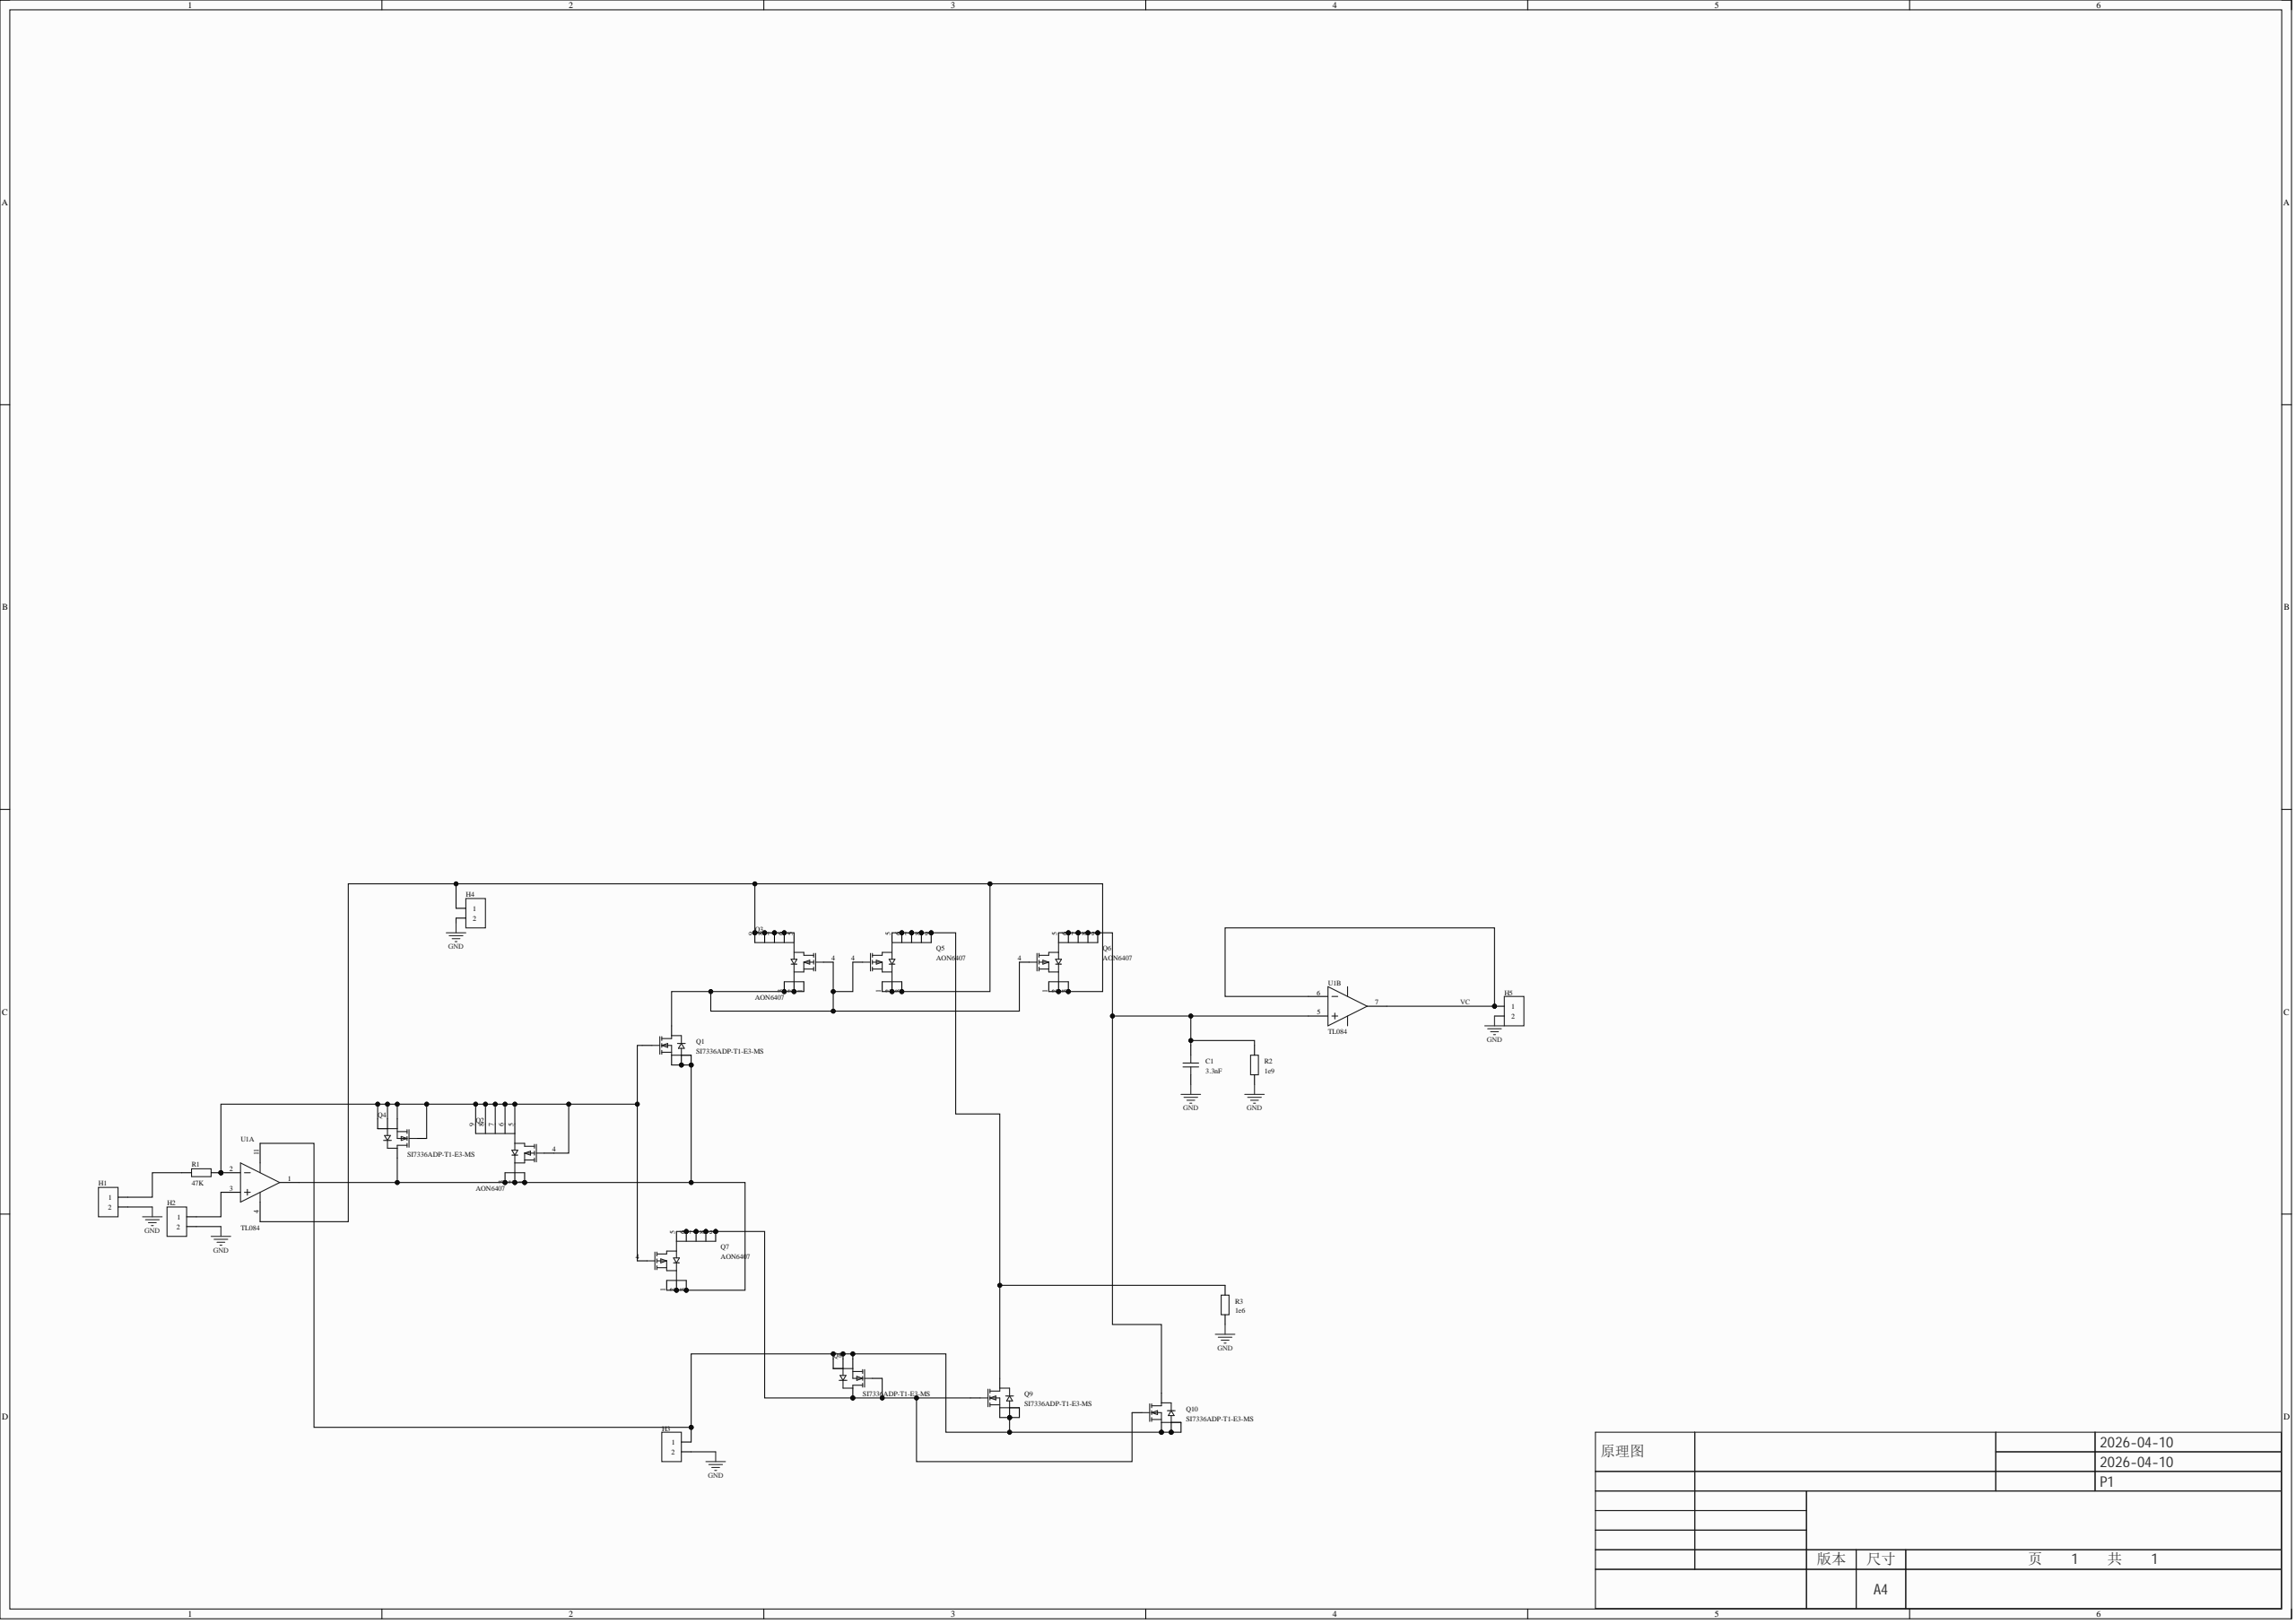Circuit board | Altium Designer | 20 parts | 12 nets
Bill of materials:
Comment,Description,Designator,Footprint,LibRef,Quantity
"3.3nF","","C1","C0805","CAP_0805","1"
"","","H1, H2, H3, H4, H5","HDR-TH_2P-P2.54-V-F","HDR-F_2.54_1x2P","5"
"SI7336ADP-T1-E3-MS","","Q1, Q4, Q8, Q9, Q10","TDSON-8_L5.9-W5.2-P1.27-BL-1","SI7336ADP-T1-E3-MS","5"
"AON6407","","Q2, Q3, Q5, Q6, Q7","PDFN-8_L4.9-W5.8-P1.27-LS6.1-BL","AON6407","5"
"47K","","R1","R0805","Res_0805","1"
"1e9","","R2","R0805","Res_0805","1"
"1e6","","R3","R0805","Res_0805","1"
"TL084","","U1","SOP-14_L8.6-W3.9-P1.27-LS6.0-BL","TL084","1"
Netlist (Protel format):
[
C1
C0805
3.3nF



]
[
H1
HDR-TH_2P-P2.54-V-F




]
[
H2
HDR-TH_2P-P2.54-V-F




]
[
H3
HDR-TH_2P-P2.54-V-F




]
[
H4
HDR-TH_2P-P2.54-V-F




]
[
H5
HDR-TH_2P-P2.54-V-F




]
[
Q1
TDSON-8_L5.9-W5.2-P1.27-BL-1
SI7336ADP-T1-E3-MS



]
[
Q2
PDFN-8_L4.9-W5.8-P1.27-LS6.1-BL
AON6407



]
[
Q3
PDFN-8_L4.9-W5.8-P1.27-LS6.1-BL
AON6407



]
[
Q4
TDSON-8_L5.9-W5.2-P1.27-BL-1
SI7336ADP-T1-E3-MS



]
[
Q5
PDFN-8_L4.9-W5.8-P1.27-LS6.1-BL
AON6407



]
[
Q6
PDFN-8_L4.9-W5.8-P1.27-LS6.1-BL
AON6407



]
[
Q7
PDFN-8_L4.9-W5.8-P1.27-LS6.1-BL
AON6407



]
[
Q8
TDSON-8_L5.9-W5.2-P1.27-BL-1
SI7336ADP-T1-E3-MS



]
[
Q9
TDSON-8_L5.9-W5.2-P1.27-BL-1
SI7336ADP-T1-E3-MS



]
[
Q10
TDSON-8_L5.9-W5.2-P1.27-BL-1
SI7336ADP-T1-E3-MS



]
[
R1
R0805
47K



]
[
R2
R0805
1e9



]
[
R3
R0805
1e6



]
[
U1
SOP-14_L8.6-W3.9-P1.27-LS6.0-BL
TL084



]
(
VC
H5-1
U1-6
U1-7
)
(
NetQ7_5
Q7-5
Q7-6
Q7-7
Q7-8
Q7-9
Q8-4
Q8-5
Q9-4
Q10-4
)
(
NetQ5_5
Q5-5
Q5-6
Q5-7
Q5-8
Q5-9
Q9-5
R3-2
)
(
NetQ1_5
Q1-5
Q3-1
Q3-2
Q3-3
Q3-4
Q5-4
Q6-4
)
(
NetQ1_4
Q1-4
Q2-4
Q2-5
Q2-6
Q2-7
Q2-8
Q2-9
Q4-1
Q4-2
Q4-3
Q4-4
Q7-4
R1-2
U1-2
)
(
NetQ1_1
Q1-1
Q1-2
Q1-3
Q2-1
Q2-2
Q2-3
Q4-5
Q7-1
Q7-2
Q7-3
U1-1
)
(
NetH4_1
H4-1
Q3-5
Q3-6
Q3-7
Q3-8
Q3-9
Q5-1
Q5-2
Q5-3
Q6-1
Q6-2
Q6-3
U1-4
)
(
NetH3_1
H3-1
Q8-1
Q8-2
Q8-3
Q9-1
Q9-2
Q9-3
Q10-1
Q10-2
Q10-3
U1-11
)
(
NetH2_1
H2-1
U1-3
)
(
NetH1_1
H1-1
R1-1
)
(
NetC1_2
C1-2
Q6-5
Q6-6
Q6-7
Q6-8
Q6-9
Q10-5
R2-2
U1-5
)
(
GND
C1-1
H1-2
H2-2
H3-2
H4-2
H5-2
R2-1
R3-1
)